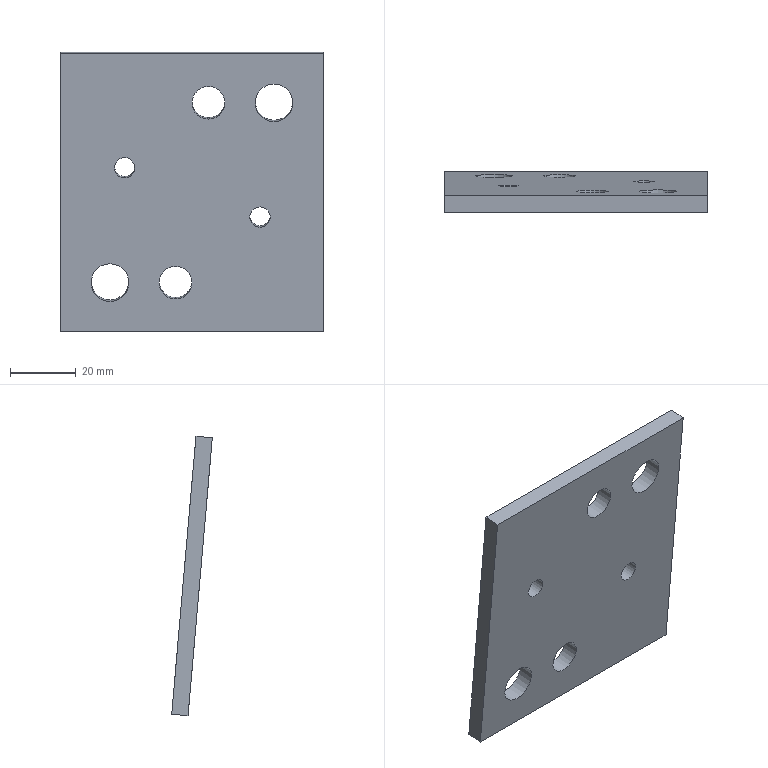Part | NX | features solid 2 | 1 solid | 12 faces | box 80 x 12.389 x 85.112 mm | volume 31874 mm3 | plane 6 | cylinder 6 | commonest cylinder face diameters 6.2 x2 10 x2 11.5 x2
STEP:
#1=CARTESIAN_POINT('',(208.,138.087,13.197));
#2=VERTEX_POINT('',#1);
#3=CARTESIAN_POINT('',(128.,138.087,13.197));
#4=VERTEX_POINT('',#3);
#5=CARTESIAN_POINT('',(208.,138.087,13.197));
#6=DIRECTION('',(-1.,0.,0.));
#7=VECTOR('',#6,1000.);
#8=LINE('',#5,#7);
#9=EDGE_CURVE('',#2,#4,#8,.T.);
#10=ORIENTED_EDGE('',*,*,#9,.F.);
#11=CARTESIAN_POINT('',(208.,143.068,13.633));
#12=VERTEX_POINT('',#11);
#13=CARTESIAN_POINT('',(208.,143.068,13.633));
#14=DIRECTION('',(0.,-0.9962,-0.08716));
#15=VECTOR('',#14,1000.);
#16=LINE('',#13,#15);
#17=EDGE_CURVE('',#12,#2,#16,.T.);
#18=ORIENTED_EDGE('',*,*,#17,.F.);
#19=CARTESIAN_POINT('',(128.,143.068,13.633));
#20=VERTEX_POINT('',#19);
#21=CARTESIAN_POINT('',(208.,143.068,13.633));
#22=DIRECTION('',(-1.,0.,0.));
#23=VECTOR('',#22,1000.);
#24=LINE('',#21,#23);
#25=EDGE_CURVE('',#12,#20,#24,.T.);
#26=ORIENTED_EDGE('',*,*,#25,.T.);
#27=CARTESIAN_POINT('',(128.,207.821,19.298));
#28=DIRECTION('',(0.,-0.9962,-0.08716));
#29=VECTOR('',#28,1000.);
#30=LINE('',#27,#29);
#31=EDGE_CURVE('',#20,#4,#30,.T.);
#32=ORIENTED_EDGE('',*,*,#31,.T.);
#33=EDGE_LOOP('',(#10,#18,#26,#32));
#34=FACE_BOUND('',#33,.T.);
#35=CARTESIAN_POINT('',(208.,143.068,13.633));
#36=DIRECTION('',(0.,0.08716,-0.9962));
#37=DIRECTION('',(0.,0.9962,0.08716));
#38=AXIS2_PLACEMENT_3D('',#35,#36,#37);
#39=PLANE('',#38);
#40=ADVANCED_FACE('',(#34),#39,.F.);
#41=CARTESIAN_POINT('',(128.,145.495,-71.479));
#42=VERTEX_POINT('',#41);
#43=CARTESIAN_POINT('',(128.,137.967,14.563));
#44=DIRECTION('',(0.,-0.08716,0.9962));
#45=VECTOR('',#44,1000.);
#46=LINE('',#43,#45);
#47=EDGE_CURVE('',#42,#4,#46,.T.);
#48=ORIENTED_EDGE('',*,*,#47,.T.);
#49=ORIENTED_EDGE('',*,*,#31,.F.);
#50=CARTESIAN_POINT('',(128.,150.476,-71.044));
#51=VERTEX_POINT('',#50);
#52=CARTESIAN_POINT('',(128.,142.948,14.999));
#53=DIRECTION('',(0.,-0.08716,0.9962));
#54=VECTOR('',#53,1000.);
#55=LINE('',#52,#54);
#56=EDGE_CURVE('',#51,#20,#55,.T.);
#57=ORIENTED_EDGE('',*,*,#56,.F.);
#58=CARTESIAN_POINT('',(128.,215.23,-65.379));
#59=DIRECTION('',(0.,-0.9962,-0.08716));
#60=VECTOR('',#59,1000.);
#61=LINE('',#58,#60);
#62=EDGE_CURVE('',#51,#42,#61,.T.);
#63=ORIENTED_EDGE('',*,*,#62,.T.);
#64=EDGE_LOOP('',(#48,#49,#57,#63));
#65=FACE_BOUND('',#64,.T.);
#66=CARTESIAN_POINT('',(128.,212.353,-32.502));
#67=DIRECTION('',(-1.,0.,0.));
#68=DIRECTION('',(0.,0.9962,0.08716));
#69=AXIS2_PLACEMENT_3D('',#66,#67,#68);
#70=PLANE('',#69);
#71=ADVANCED_FACE('',(#65),#70,.T.);
#72=CARTESIAN_POINT('',(208.,145.495,-71.479));
#73=VERTEX_POINT('',#72);
#74=CARTESIAN_POINT('',(171.,145.495,-71.479));
#75=DIRECTION('',(1.,0.,0.));
#76=VECTOR('',#75,1000.);
#77=LINE('',#74,#76);
#78=EDGE_CURVE('',#42,#73,#77,.T.);
#79=ORIENTED_EDGE('',*,*,#78,.F.);
#80=ORIENTED_EDGE('',*,*,#62,.F.);
#81=CARTESIAN_POINT('',(208.,150.476,-71.044));
#82=VERTEX_POINT('',#81);
#83=CARTESIAN_POINT('',(171.,150.476,-71.044));
#84=DIRECTION('',(1.,0.,0.));
#85=VECTOR('',#84,1000.);
#86=LINE('',#83,#85);
#87=EDGE_CURVE('',#51,#82,#86,.T.);
#88=ORIENTED_EDGE('',*,*,#87,.T.);
#89=CARTESIAN_POINT('',(208.,279.982,-59.713));
#90=DIRECTION('',(0.,-0.9962,-0.08716));
#91=VECTOR('',#90,1000.);
#92=LINE('',#89,#91);
#93=EDGE_CURVE('',#82,#73,#92,.T.);
#94=ORIENTED_EDGE('',*,*,#93,.T.);
#95=EDGE_LOOP('',(#79,#80,#88,#94));
#96=FACE_BOUND('',#95,.T.);
#97=CARTESIAN_POINT('',(171.,279.982,-59.713));
#98=DIRECTION('',(0.,0.08716,-0.9962));
#99=DIRECTION('',(-1.,0.,0.));
#100=AXIS2_PLACEMENT_3D('',#97,#98,#99);
#101=PLANE('',#100);
#102=ADVANCED_FACE('',(#96),#101,.T.);
#103=CARTESIAN_POINT('',(208.,137.967,14.563));
#104=DIRECTION('',(0.,0.08716,-0.9962));
#105=VECTOR('',#104,1000.);
#106=LINE('',#103,#105);
#107=EDGE_CURVE('',#2,#73,#106,.T.);
#108=ORIENTED_EDGE('',*,*,#107,.T.);
#109=ORIENTED_EDGE('',*,*,#93,.F.);
#110=CARTESIAN_POINT('',(208.,142.948,14.999));
#111=DIRECTION('',(0.,0.08716,-0.9962));
#112=VECTOR('',#111,1000.);
#113=LINE('',#110,#112);
#114=EDGE_CURVE('',#12,#82,#113,.T.);
#115=ORIENTED_EDGE('',*,*,#114,.F.);
#116=ORIENTED_EDGE('',*,*,#17,.T.);
#117=EDGE_LOOP('',(#108,#109,#115,#116));
#118=FACE_BOUND('',#117,.T.);
#119=CARTESIAN_POINT('',(208.,212.353,-32.502));
#120=DIRECTION('',(1.,0.,0.));
#121=DIRECTION('',(0.,-0.9962,-0.08716));
#122=AXIS2_PLACEMENT_3D('',#119,#120,#121);
#123=PLANE('',#122);
#124=ADVANCED_FACE('',(#118),#123,.T.);
#125=CARTESIAN_POINT('',(188.737,147.151,-33.036));
#126=VERTEX_POINT('',#125);
#127=CARTESIAN_POINT('',(188.737,147.421,-36.125));
#128=DIRECTION('',(0.,0.9962,0.08716));
#129=DIRECTION('',(0.,-0.08716,0.9962));
#130=AXIS2_PLACEMENT_3D('',#127,#128,#129);
#131=CIRCLE('',#130,3.1);
#132=EDGE_CURVE('',#126,#126,#131,.F.);
#133=ORIENTED_EDGE('',*,*,#132,.T.);
#134=EDGE_LOOP('',(#133));
#135=FACE_BOUND('',#134,.T.);
#136=CARTESIAN_POINT('',(147.466,145.839,-18.034));
#137=VERTEX_POINT('',#136);
#138=CARTESIAN_POINT('',(147.466,146.109,-21.122));
#139=DIRECTION('',(0.,0.9962,0.08716));
#140=DIRECTION('',(0.,-0.08716,0.9962));
#141=AXIS2_PLACEMENT_3D('',#138,#139,#140);
#142=CIRCLE('',#141,3.1);
#143=EDGE_CURVE('',#137,#137,#142,.F.);
#144=ORIENTED_EDGE('',*,*,#143,.T.);
#145=EDGE_LOOP('',(#144));
#146=FACE_BOUND('',#145,.T.);
#147=CARTESIAN_POINT('',(193.,143.874,4.418));
#148=VERTEX_POINT('',#147);
#149=CARTESIAN_POINT('',(193.,144.375,-1.31));
#150=DIRECTION('',(0.,0.9962,0.08716));
#151=DIRECTION('',(0.,-0.08716,0.9962));
#152=AXIS2_PLACEMENT_3D('',#149,#150,#151);
#153=CIRCLE('',#152,5.75);
#154=EDGE_CURVE('',#148,#148,#153,.F.);
#155=ORIENTED_EDGE('',*,*,#154,.T.);
#156=EDGE_LOOP('',(#155));
#157=FACE_BOUND('',#156,.T.);
#158=CARTESIAN_POINT('',(173.,143.94,3.671));
#159=VERTEX_POINT('',#158);
#160=CARTESIAN_POINT('',(173.,144.375,-1.31));
#161=DIRECTION('',(0.,0.9962,0.08716));
#162=DIRECTION('',(0.,-0.08716,0.9962));
#163=AXIS2_PLACEMENT_3D('',#160,#161,#162);
#164=CIRCLE('',#163,5.);
#165=EDGE_CURVE('',#159,#159,#164,.F.);
#166=ORIENTED_EDGE('',*,*,#165,.T.);
#167=EDGE_LOOP('',(#166));
#168=FACE_BOUND('',#167,.T.);
#169=CARTESIAN_POINT('',(163.,148.733,-51.12));
#170=VERTEX_POINT('',#169);
#171=CARTESIAN_POINT('',(163.,149.169,-56.101));
#172=DIRECTION('',(0.,0.9962,0.08716));
#173=DIRECTION('',(0.,-0.08716,0.9962));
#174=AXIS2_PLACEMENT_3D('',#171,#172,#173);
#175=CIRCLE('',#174,5.);
#176=EDGE_CURVE('',#170,#170,#175,.F.);
#177=ORIENTED_EDGE('',*,*,#176,.T.);
#178=EDGE_LOOP('',(#177));
#179=FACE_BOUND('',#178,.T.);
#180=CARTESIAN_POINT('',(143.,148.668,-50.373));
#181=VERTEX_POINT('',#180);
#182=CARTESIAN_POINT('',(143.,149.169,-56.101));
#183=DIRECTION('',(0.,0.9962,0.08716));
#184=DIRECTION('',(0.,-0.08716,0.9962));
#185=AXIS2_PLACEMENT_3D('',#182,#183,#184);
#186=CIRCLE('',#185,5.75);
#187=EDGE_CURVE('',#181,#181,#186,.F.);
#188=ORIENTED_EDGE('',*,*,#187,.T.);
#189=EDGE_LOOP('',(#188));
#190=FACE_BOUND('',#189,.T.);
#191=ORIENTED_EDGE('',*,*,#25,.F.);
#192=ORIENTED_EDGE('',*,*,#114,.T.);
#193=ORIENTED_EDGE('',*,*,#87,.F.);
#194=ORIENTED_EDGE('',*,*,#56,.T.);
#195=EDGE_LOOP('',(#191,#192,#193,#194));
#196=FACE_BOUND('',#195,.T.);
#197=CARTESIAN_POINT('',(208.,142.948,14.999));
#198=DIRECTION('',(0.,0.9962,0.08716));
#199=DIRECTION('',(-1.,0.,0.));
#200=AXIS2_PLACEMENT_3D('',#197,#198,#199);
#201=PLANE('',#200);
#202=ADVANCED_FACE('',(#135,#146,#157,#168,#179,#190,#196),#201,.T.);
#203=CARTESIAN_POINT('',(188.737,142.17,-33.472));
#204=VERTEX_POINT('',#203);
#205=CARTESIAN_POINT('',(188.737,142.44,-36.56));
#206=DIRECTION('',(0.,0.9962,0.08716));
#207=DIRECTION('',(0.,-0.08716,0.9962));
#208=AXIS2_PLACEMENT_3D('',#205,#206,#207);
#209=CIRCLE('',#208,3.1);
#210=EDGE_CURVE('',#204,#204,#209,.F.);
#211=ORIENTED_EDGE('',*,*,#210,.F.);
#212=EDGE_LOOP('',(#211));
#213=FACE_BOUND('',#212,.T.);
#214=CARTESIAN_POINT('',(147.466,140.858,-18.47));
#215=VERTEX_POINT('',#214);
#216=CARTESIAN_POINT('',(147.466,141.128,-21.558));
#217=DIRECTION('',(0.,0.9962,0.08716));
#218=DIRECTION('',(0.,-0.08716,0.9962));
#219=AXIS2_PLACEMENT_3D('',#216,#217,#218);
#220=CIRCLE('',#219,3.1);
#221=EDGE_CURVE('',#215,#215,#220,.F.);
#222=ORIENTED_EDGE('',*,*,#221,.F.);
#223=EDGE_LOOP('',(#222));
#224=FACE_BOUND('',#223,.T.);
#225=CARTESIAN_POINT('',(193.,138.893,3.982));
#226=VERTEX_POINT('',#225);
#227=CARTESIAN_POINT('',(193.,139.394,-1.746));
#228=DIRECTION('',(0.,0.9962,0.08716));
#229=DIRECTION('',(0.,-0.08716,0.9962));
#230=AXIS2_PLACEMENT_3D('',#227,#228,#229);
#231=CIRCLE('',#230,5.75);
#232=EDGE_CURVE('',#226,#226,#231,.F.);
#233=ORIENTED_EDGE('',*,*,#232,.F.);
#234=EDGE_LOOP('',(#233));
#235=FACE_BOUND('',#234,.T.);
#236=CARTESIAN_POINT('',(173.,138.959,3.235));
#237=VERTEX_POINT('',#236);
#238=CARTESIAN_POINT('',(173.,139.394,-1.746));
#239=DIRECTION('',(0.,0.9962,0.08716));
#240=DIRECTION('',(0.,-0.08716,0.9962));
#241=AXIS2_PLACEMENT_3D('',#238,#239,#240);
#242=CIRCLE('',#241,5.);
#243=EDGE_CURVE('',#237,#237,#242,.F.);
#244=ORIENTED_EDGE('',*,*,#243,.F.);
#245=EDGE_LOOP('',(#244));
#246=FACE_BOUND('',#245,.T.);
#247=CARTESIAN_POINT('',(163.,143.752,-51.556));
#248=VERTEX_POINT('',#247);
#249=CARTESIAN_POINT('',(163.,144.188,-56.537));
#250=DIRECTION('',(0.,0.9962,0.08716));
#251=DIRECTION('',(0.,-0.08716,0.9962));
#252=AXIS2_PLACEMENT_3D('',#249,#250,#251);
#253=CIRCLE('',#252,5.);
#254=EDGE_CURVE('',#248,#248,#253,.F.);
#255=ORIENTED_EDGE('',*,*,#254,.F.);
#256=EDGE_LOOP('',(#255));
#257=FACE_BOUND('',#256,.T.);
#258=CARTESIAN_POINT('',(143.,143.687,-50.808));
#259=VERTEX_POINT('',#258);
#260=CARTESIAN_POINT('',(143.,144.188,-56.537));
#261=DIRECTION('',(0.,0.9962,0.08716));
#262=DIRECTION('',(0.,-0.08716,0.9962));
#263=AXIS2_PLACEMENT_3D('',#260,#261,#262);
#264=CIRCLE('',#263,5.75);
#265=EDGE_CURVE('',#259,#259,#264,.F.);
#266=ORIENTED_EDGE('',*,*,#265,.F.);
#267=EDGE_LOOP('',(#266));
#268=FACE_BOUND('',#267,.T.);
#269=ORIENTED_EDGE('',*,*,#9,.T.);
#270=ORIENTED_EDGE('',*,*,#47,.F.);
#271=ORIENTED_EDGE('',*,*,#78,.T.);
#272=ORIENTED_EDGE('',*,*,#107,.F.);
#273=EDGE_LOOP('',(#269,#270,#271,#272));
#274=FACE_BOUND('',#273,.T.);
#275=CARTESIAN_POINT('',(208.,137.967,14.563));
#276=DIRECTION('',(0.,0.9962,0.08716));
#277=DIRECTION('',(-1.,0.,0.));
#278=AXIS2_PLACEMENT_3D('',#275,#276,#277);
#279=PLANE('',#278);
#280=ADVANCED_FACE('',(#213,#224,#235,#246,#257,#268,#274),#279,.F.);
#281=ORIENTED_EDGE('',*,*,#265,.T.);
#282=EDGE_LOOP('',(#281));
#283=FACE_BOUND('',#282,.T.);
#284=ORIENTED_EDGE('',*,*,#187,.F.);
#285=EDGE_LOOP('',(#284));
#286=FACE_BOUND('',#285,.T.);
#287=CARTESIAN_POINT('',(143.,119.283,-58.715));
#288=DIRECTION('',(0.,0.9962,0.08716));
#289=DIRECTION('',(1.,0.,0.));
#290=AXIS2_PLACEMENT_3D('',#287,#288,#289);
#291=CYLINDRICAL_SURFACE('',#290,5.75);
#292=ADVANCED_FACE('',(#283,#286),#291,.F.);
#293=ORIENTED_EDGE('',*,*,#254,.T.);
#294=EDGE_LOOP('',(#293));
#295=FACE_BOUND('',#294,.T.);
#296=ORIENTED_EDGE('',*,*,#176,.F.);
#297=EDGE_LOOP('',(#296));
#298=FACE_BOUND('',#297,.T.);
#299=CARTESIAN_POINT('',(163.,119.283,-58.715));
#300=DIRECTION('',(0.,0.9962,0.08716));
#301=DIRECTION('',(1.,0.,0.));
#302=AXIS2_PLACEMENT_3D('',#299,#300,#301);
#303=CYLINDRICAL_SURFACE('',#302,5.);
#304=ADVANCED_FACE('',(#295,#298),#303,.F.);
#305=ORIENTED_EDGE('',*,*,#243,.T.);
#306=EDGE_LOOP('',(#305));
#307=FACE_BOUND('',#306,.T.);
#308=ORIENTED_EDGE('',*,*,#165,.F.);
#309=EDGE_LOOP('',(#308));
#310=FACE_BOUND('',#309,.T.);
#311=CARTESIAN_POINT('',(173.,114.489,-3.925));
#312=DIRECTION('',(0.,0.9962,0.08716));
#313=DIRECTION('',(1.,0.,0.));
#314=AXIS2_PLACEMENT_3D('',#311,#312,#313);
#315=CYLINDRICAL_SURFACE('',#314,5.);
#316=ADVANCED_FACE('',(#307,#310),#315,.F.);
#317=ORIENTED_EDGE('',*,*,#232,.T.);
#318=EDGE_LOOP('',(#317));
#319=FACE_BOUND('',#318,.T.);
#320=ORIENTED_EDGE('',*,*,#154,.F.);
#321=EDGE_LOOP('',(#320));
#322=FACE_BOUND('',#321,.T.);
#323=CARTESIAN_POINT('',(193.,114.489,-3.925));
#324=DIRECTION('',(0.,0.9962,0.08716));
#325=DIRECTION('',(1.,0.,0.));
#326=AXIS2_PLACEMENT_3D('',#323,#324,#325);
#327=CYLINDRICAL_SURFACE('',#326,5.75);
#328=ADVANCED_FACE('',(#319,#322),#327,.F.);
#329=ORIENTED_EDGE('',*,*,#221,.T.);
#330=EDGE_LOOP('',(#329));
#331=FACE_BOUND('',#330,.T.);
#332=ORIENTED_EDGE('',*,*,#143,.F.);
#333=EDGE_LOOP('',(#332));
#334=FACE_BOUND('',#333,.T.);
#335=CARTESIAN_POINT('',(147.466,16.603,-32.453));
#336=DIRECTION('',(0.,0.9962,0.08716));
#337=DIRECTION('',(1.,0.,0.));
#338=AXIS2_PLACEMENT_3D('',#335,#336,#337);
#339=CYLINDRICAL_SURFACE('',#338,3.1);
#340=ADVANCED_FACE('',(#331,#334),#339,.F.);
#341=ORIENTED_EDGE('',*,*,#210,.T.);
#342=EDGE_LOOP('',(#341));
#343=FACE_BOUND('',#342,.T.);
#344=ORIENTED_EDGE('',*,*,#132,.F.);
#345=EDGE_LOOP('',(#344));
#346=FACE_BOUND('',#345,.T.);
#347=CARTESIAN_POINT('',(188.737,-47.833,-53.207));
#348=DIRECTION('',(0.,0.9962,0.08716));
#349=DIRECTION('',(1.,0.,0.));
#350=AXIS2_PLACEMENT_3D('',#347,#348,#349);
#351=CYLINDRICAL_SURFACE('',#350,3.1);
#352=ADVANCED_FACE('',(#343,#346),#351,.F.);
#353=CLOSED_SHELL('',(#40,#71,#102,#124,#202,#280,#292,#304,#316,#328,#340,#352));
#354=MANIFOLD_SOLID_BREP('',#353);
#355=(LENGTH_UNIT()NAMED_UNIT(*)SI_UNIT(.MILLI.,.METRE.));
#356=UNCERTAINTY_MEASURE_WITH_UNIT(LENGTH_MEASURE(0.00001),#355,'','');
#357=(NAMED_UNIT(*)PLANE_ANGLE_UNIT()SI_UNIT($,.RADIAN.));
#358=(NAMED_UNIT(*)SI_UNIT($,.STERADIAN.)SOLID_ANGLE_UNIT());
#359=(GEOMETRIC_REPRESENTATION_CONTEXT(3)GLOBAL_UNCERTAINTY_ASSIGNED_CONTEXT((#356))GLOBAL_UNIT_ASSIGNED_CONTEXT((#355,#357,#358))REPRESENTATION_CONTEXT('',''));
#360=ADVANCED_BREP_SHAPE_REPRESENTATION('',(#354),#359);